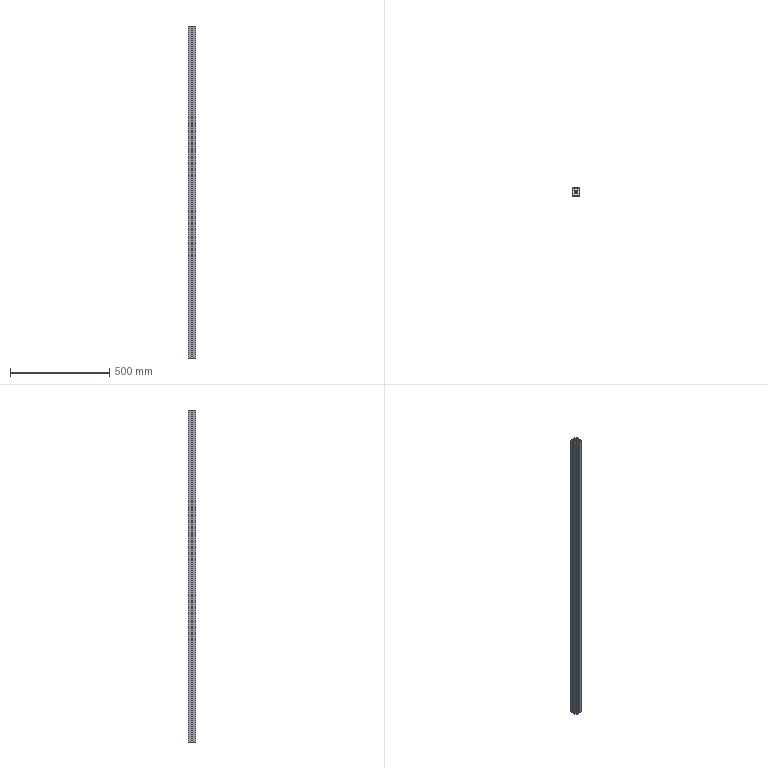Part | STEP file | 40_40_1590_1-2 | 1 solid | 64 faces | box 40 x 40 x 1670 mm | volume 876321 mm3 | plane 62 | cylinder 2 | commonest cylinder face diameters 6.8 x2